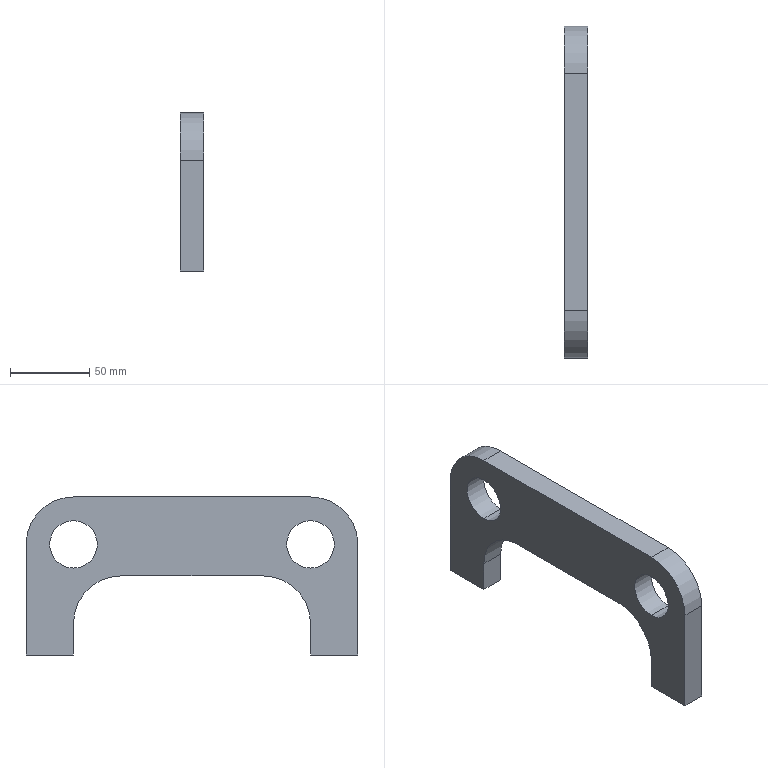Part | SolidWorks | features Cut 1, Extrusion 1 | 1 solid | 18 faces | box 15 x 210 x 100 mm | volume 181294 mm3 | plane 10 | cylinder 8 | commonest cylinder face diameters 30 x4 60 x4
STEP:
#1=CARTESIAN_POINT('',(-215.412,-13.,55.));
#2=VERTEX_POINT('',#1);
#3=CARTESIAN_POINT('',(-215.412,-13.,85.));
#4=VERTEX_POINT('',#3);
#5=CARTESIAN_POINT('',(-215.412,-13.,70.));
#6=DIRECTION('',(-1.,0.,0.));
#7=DIRECTION('',(0.,0.,1.));
#8=AXIS2_PLACEMENT_3D('',#5,#6,#7);
#9=CIRCLE('',#8,15.);
#10=EDGE_CURVE('',#2,#4,#9,.T.);
#11=ORIENTED_EDGE('',*,*,#10,.F.);
#12=CARTESIAN_POINT('',(-230.412,-13.,55.));
#13=VERTEX_POINT('',#12);
#14=CARTESIAN_POINT('',(-215.412,-13.,55.));
#15=DIRECTION('',(-1.,0.,0.));
#16=VECTOR('',#15,1000.);
#17=LINE('',#14,#16);
#18=EDGE_CURVE('',#2,#13,#17,.T.);
#19=ORIENTED_EDGE('',*,*,#18,.T.);
#20=CARTESIAN_POINT('',(-230.412,-13.,85.));
#21=VERTEX_POINT('',#20);
#22=CARTESIAN_POINT('',(-230.412,-13.,70.));
#23=DIRECTION('',(-1.,0.,0.));
#24=DIRECTION('',(0.,0.,1.));
#25=AXIS2_PLACEMENT_3D('',#22,#23,#24);
#26=CIRCLE('',#25,15.);
#27=EDGE_CURVE('',#13,#21,#26,.T.);
#28=ORIENTED_EDGE('',*,*,#27,.T.);
#29=CARTESIAN_POINT('',(-215.412,-13.,85.));
#30=DIRECTION('',(-1.,0.,0.));
#31=VECTOR('',#30,1000.);
#32=LINE('',#29,#31);
#33=EDGE_CURVE('',#4,#21,#32,.T.);
#34=ORIENTED_EDGE('',*,*,#33,.F.);
#35=EDGE_LOOP('',(#11,#19,#28,#34));
#36=FACE_OUTER_BOUND('',#35,.T.);
#37=CARTESIAN_POINT('',(-215.412,-13.,70.));
#38=DIRECTION('',(-1.,0.,0.));
#39=DIRECTION('',(0.,0.,1.));
#40=AXIS2_PLACEMENT_3D('',#37,#38,#39);
#41=CYLINDRICAL_SURFACE('',#40,15.);
#42=ADVANCED_FACE('',(#36),#41,.F.);
#43=CARTESIAN_POINT('',(-215.412,137.,55.));
#44=VERTEX_POINT('',#43);
#45=CARTESIAN_POINT('',(-215.412,137.,85.));
#46=VERTEX_POINT('',#45);
#47=CARTESIAN_POINT('',(-215.412,137.,70.));
#48=DIRECTION('',(-1.,0.,0.));
#49=DIRECTION('',(0.,0.,1.));
#50=AXIS2_PLACEMENT_3D('',#47,#48,#49);
#51=CIRCLE('',#50,15.);
#52=EDGE_CURVE('',#44,#46,#51,.T.);
#53=ORIENTED_EDGE('',*,*,#52,.F.);
#54=CARTESIAN_POINT('',(-230.412,137.,55.));
#55=VERTEX_POINT('',#54);
#56=CARTESIAN_POINT('',(-215.412,137.,55.));
#57=DIRECTION('',(-1.,0.,0.));
#58=VECTOR('',#57,1000.);
#59=LINE('',#56,#58);
#60=EDGE_CURVE('',#44,#55,#59,.T.);
#61=ORIENTED_EDGE('',*,*,#60,.T.);
#62=CARTESIAN_POINT('',(-230.412,137.,85.));
#63=VERTEX_POINT('',#62);
#64=CARTESIAN_POINT('',(-230.412,137.,70.));
#65=DIRECTION('',(-1.,0.,0.));
#66=DIRECTION('',(0.,0.,1.));
#67=AXIS2_PLACEMENT_3D('',#64,#65,#66);
#68=CIRCLE('',#67,15.);
#69=EDGE_CURVE('',#55,#63,#68,.T.);
#70=ORIENTED_EDGE('',*,*,#69,.T.);
#71=CARTESIAN_POINT('',(-215.412,137.,85.));
#72=DIRECTION('',(-1.,0.,0.));
#73=VECTOR('',#72,1000.);
#74=LINE('',#71,#73);
#75=EDGE_CURVE('',#46,#63,#74,.T.);
#76=ORIENTED_EDGE('',*,*,#75,.F.);
#77=EDGE_LOOP('',(#53,#61,#70,#76));
#78=FACE_OUTER_BOUND('',#77,.T.);
#79=CARTESIAN_POINT('',(-215.412,137.,70.));
#80=DIRECTION('',(-1.,0.,0.));
#81=DIRECTION('',(0.,0.,1.));
#82=AXIS2_PLACEMENT_3D('',#79,#80,#81);
#83=CYLINDRICAL_SURFACE('',#82,15.);
#84=ADVANCED_FACE('',(#78),#83,.F.);
#85=CARTESIAN_POINT('',(-230.412,-13.,0.));
#86=VERTEX_POINT('',#85);
#87=CARTESIAN_POINT('',(-230.412,-43.,0.));
#88=VERTEX_POINT('',#87);
#89=CARTESIAN_POINT('',(-230.412,-13.,0.));
#90=DIRECTION('',(0.,-1.,0.));
#91=VECTOR('',#90,1000.);
#92=LINE('',#89,#91);
#93=EDGE_CURVE('',#86,#88,#92,.T.);
#94=ORIENTED_EDGE('',*,*,#93,.F.);
#95=CARTESIAN_POINT('',(-215.412,-13.,0.));
#96=VERTEX_POINT('',#95);
#97=CARTESIAN_POINT('',(-463.006,-13.,0.));
#98=DIRECTION('',(1.,0.,0.));
#99=VECTOR('',#98,1000.);
#100=LINE('',#97,#99);
#101=EDGE_CURVE('',#86,#96,#100,.T.);
#102=ORIENTED_EDGE('',*,*,#101,.T.);
#103=CARTESIAN_POINT('',(-215.412,-43.,0.));
#104=VERTEX_POINT('',#103);
#105=CARTESIAN_POINT('',(-215.412,-13.,0.));
#106=DIRECTION('',(0.,-1.,0.));
#107=VECTOR('',#106,1000.);
#108=LINE('',#105,#107);
#109=EDGE_CURVE('',#96,#104,#108,.T.);
#110=ORIENTED_EDGE('',*,*,#109,.T.);
#111=CARTESIAN_POINT('',(-463.006,-43.,0.));
#112=DIRECTION('',(1.,0.,0.));
#113=VECTOR('',#112,1000.);
#114=LINE('',#111,#113);
#115=EDGE_CURVE('',#88,#104,#114,.T.);
#116=ORIENTED_EDGE('',*,*,#115,.F.);
#117=EDGE_LOOP('',(#94,#102,#110,#116));
#118=FACE_OUTER_BOUND('',#117,.T.);
#119=CARTESIAN_POINT('',(-463.006,-13.,0.));
#120=DIRECTION('',(0.,0.,1.));
#121=DIRECTION('',(1.,0.,0.));
#122=AXIS2_PLACEMENT_3D('',#119,#120,#121);
#123=PLANE('',#122);
#124=ADVANCED_FACE('',(#118),#123,.F.);
#125=CARTESIAN_POINT('',(-230.412,-43.,70.));
#126=VERTEX_POINT('',#125);
#127=CARTESIAN_POINT('',(-230.412,-43.,70.));
#128=DIRECTION('',(0.,0.,1.));
#129=VECTOR('',#128,1000.);
#130=LINE('',#127,#129);
#131=EDGE_CURVE('',#88,#126,#130,.T.);
#132=ORIENTED_EDGE('',*,*,#131,.F.);
#133=ORIENTED_EDGE('',*,*,#115,.T.);
#134=CARTESIAN_POINT('',(-215.412,-43.,70.));
#135=VERTEX_POINT('',#134);
#136=CARTESIAN_POINT('',(-215.412,-43.,70.));
#137=DIRECTION('',(0.,0.,1.));
#138=VECTOR('',#137,1000.);
#139=LINE('',#136,#138);
#140=EDGE_CURVE('',#104,#135,#139,.T.);
#141=ORIENTED_EDGE('',*,*,#140,.T.);
#142=CARTESIAN_POINT('',(-463.006,-43.,70.));
#143=DIRECTION('',(1.,0.,0.));
#144=VECTOR('',#143,1000.);
#145=LINE('',#142,#144);
#146=EDGE_CURVE('',#126,#135,#145,.T.);
#147=ORIENTED_EDGE('',*,*,#146,.F.);
#148=EDGE_LOOP('',(#132,#133,#141,#147));
#149=FACE_OUTER_BOUND('',#148,.T.);
#150=CARTESIAN_POINT('',(-463.006,-43.,70.));
#151=DIRECTION('',(0.,1.,0.));
#152=DIRECTION('',(0.,0.,1.));
#153=AXIS2_PLACEMENT_3D('',#150,#151,#152);
#154=PLANE('',#153);
#155=ADVANCED_FACE('',(#149),#154,.F.);
#156=CARTESIAN_POINT('',(-230.412,-13.,100.));
#157=VERTEX_POINT('',#156);
#158=CARTESIAN_POINT('',(-230.412,-13.,70.));
#159=DIRECTION('',(-1.,0.,0.));
#160=DIRECTION('',(0.,0.,1.));
#161=AXIS2_PLACEMENT_3D('',#158,#159,#160);
#162=CIRCLE('',#161,30.);
#163=EDGE_CURVE('',#126,#157,#162,.T.);
#164=ORIENTED_EDGE('',*,*,#163,.F.);
#165=ORIENTED_EDGE('',*,*,#146,.T.);
#166=CARTESIAN_POINT('',(-215.412,-13.,100.));
#167=VERTEX_POINT('',#166);
#168=CARTESIAN_POINT('',(-215.412,-13.,70.));
#169=DIRECTION('',(-1.,0.,0.));
#170=DIRECTION('',(0.,0.,-1.));
#171=AXIS2_PLACEMENT_3D('',#168,#169,#170);
#172=CIRCLE('',#171,30.);
#173=EDGE_CURVE('',#135,#167,#172,.T.);
#174=ORIENTED_EDGE('',*,*,#173,.T.);
#175=CARTESIAN_POINT('',(-463.006,-13.,100.));
#176=DIRECTION('',(1.,0.,0.));
#177=VECTOR('',#176,1000.);
#178=LINE('',#175,#177);
#179=EDGE_CURVE('',#157,#167,#178,.T.);
#180=ORIENTED_EDGE('',*,*,#179,.F.);
#181=EDGE_LOOP('',(#164,#165,#174,#180));
#182=FACE_OUTER_BOUND('',#181,.T.);
#183=CARTESIAN_POINT('',(-463.006,-13.,70.));
#184=DIRECTION('',(1.,0.,0.));
#185=DIRECTION('',(0.,0.,-1.));
#186=AXIS2_PLACEMENT_3D('',#183,#184,#185);
#187=CYLINDRICAL_SURFACE('',#186,30.);
#188=ADVANCED_FACE('',(#182),#187,.T.);
#189=CARTESIAN_POINT('',(-230.412,137.,100.));
#190=VERTEX_POINT('',#189);
#191=CARTESIAN_POINT('',(-230.412,137.,100.));
#192=DIRECTION('',(0.,1.,0.));
#193=VECTOR('',#192,1000.);
#194=LINE('',#191,#193);
#195=EDGE_CURVE('',#157,#190,#194,.T.);
#196=ORIENTED_EDGE('',*,*,#195,.F.);
#197=ORIENTED_EDGE('',*,*,#179,.T.);
#198=CARTESIAN_POINT('',(-215.412,137.,100.));
#199=VERTEX_POINT('',#198);
#200=CARTESIAN_POINT('',(-215.412,137.,100.));
#201=DIRECTION('',(0.,1.,0.));
#202=VECTOR('',#201,1000.);
#203=LINE('',#200,#202);
#204=EDGE_CURVE('',#167,#199,#203,.T.);
#205=ORIENTED_EDGE('',*,*,#204,.T.);
#206=CARTESIAN_POINT('',(-463.006,137.,100.));
#207=DIRECTION('',(1.,0.,0.));
#208=VECTOR('',#207,1000.);
#209=LINE('',#206,#208);
#210=EDGE_CURVE('',#190,#199,#209,.T.);
#211=ORIENTED_EDGE('',*,*,#210,.F.);
#212=EDGE_LOOP('',(#196,#197,#205,#211));
#213=FACE_OUTER_BOUND('',#212,.T.);
#214=CARTESIAN_POINT('',(-463.006,137.,100.));
#215=DIRECTION('',(0.,0.,-1.));
#216=DIRECTION('',(-1.,0.,0.));
#217=AXIS2_PLACEMENT_3D('',#214,#215,#216);
#218=PLANE('',#217);
#219=ADVANCED_FACE('',(#213),#218,.F.);
#220=CARTESIAN_POINT('',(-230.412,167.,70.));
#221=VERTEX_POINT('',#220);
#222=CARTESIAN_POINT('',(-230.412,137.,70.));
#223=DIRECTION('',(-1.,0.,0.));
#224=DIRECTION('',(0.,0.,1.));
#225=AXIS2_PLACEMENT_3D('',#222,#223,#224);
#226=CIRCLE('',#225,30.);
#227=EDGE_CURVE('',#190,#221,#226,.T.);
#228=ORIENTED_EDGE('',*,*,#227,.F.);
#229=ORIENTED_EDGE('',*,*,#210,.T.);
#230=CARTESIAN_POINT('',(-215.412,167.,70.));
#231=VERTEX_POINT('',#230);
#232=CARTESIAN_POINT('',(-215.412,137.,70.));
#233=DIRECTION('',(-1.,0.,0.));
#234=DIRECTION('',(0.,0.,-1.));
#235=AXIS2_PLACEMENT_3D('',#232,#233,#234);
#236=CIRCLE('',#235,30.);
#237=EDGE_CURVE('',#199,#231,#236,.T.);
#238=ORIENTED_EDGE('',*,*,#237,.T.);
#239=CARTESIAN_POINT('',(-463.006,167.,70.));
#240=DIRECTION('',(1.,0.,0.));
#241=VECTOR('',#240,1000.);
#242=LINE('',#239,#241);
#243=EDGE_CURVE('',#221,#231,#242,.T.);
#244=ORIENTED_EDGE('',*,*,#243,.F.);
#245=EDGE_LOOP('',(#228,#229,#238,#244));
#246=FACE_OUTER_BOUND('',#245,.T.);
#247=CARTESIAN_POINT('',(-463.006,137.,70.));
#248=DIRECTION('',(1.,0.,0.));
#249=DIRECTION('',(0.,0.,-1.));
#250=AXIS2_PLACEMENT_3D('',#247,#248,#249);
#251=CYLINDRICAL_SURFACE('',#250,30.);
#252=ADVANCED_FACE('',(#246),#251,.T.);
#253=CARTESIAN_POINT('',(-230.412,167.,0.));
#254=VERTEX_POINT('',#253);
#255=CARTESIAN_POINT('',(-230.412,167.,0.));
#256=DIRECTION('',(0.,0.,-1.));
#257=VECTOR('',#256,1000.);
#258=LINE('',#255,#257);
#259=EDGE_CURVE('',#221,#254,#258,.T.);
#260=ORIENTED_EDGE('',*,*,#259,.F.);
#261=ORIENTED_EDGE('',*,*,#243,.T.);
#262=CARTESIAN_POINT('',(-215.412,167.,0.));
#263=VERTEX_POINT('',#262);
#264=CARTESIAN_POINT('',(-215.412,167.,0.));
#265=DIRECTION('',(0.,0.,-1.));
#266=VECTOR('',#265,1000.);
#267=LINE('',#264,#266);
#268=EDGE_CURVE('',#231,#263,#267,.T.);
#269=ORIENTED_EDGE('',*,*,#268,.T.);
#270=CARTESIAN_POINT('',(-463.006,167.,0.));
#271=DIRECTION('',(1.,0.,0.));
#272=VECTOR('',#271,1000.);
#273=LINE('',#270,#272);
#274=EDGE_CURVE('',#254,#263,#273,.T.);
#275=ORIENTED_EDGE('',*,*,#274,.F.);
#276=EDGE_LOOP('',(#260,#261,#269,#275));
#277=FACE_OUTER_BOUND('',#276,.T.);
#278=CARTESIAN_POINT('',(-463.006,167.,0.));
#279=DIRECTION('',(0.,-1.,0.));
#280=DIRECTION('',(1.,0.,0.));
#281=AXIS2_PLACEMENT_3D('',#278,#279,#280);
#282=PLANE('',#281);
#283=ADVANCED_FACE('',(#277),#282,.F.);
#284=CARTESIAN_POINT('',(-230.412,137.,0.));
#285=VERTEX_POINT('',#284);
#286=CARTESIAN_POINT('',(-230.412,137.,0.));
#287=DIRECTION('',(0.,-1.,0.));
#288=VECTOR('',#287,1000.);
#289=LINE('',#286,#288);
#290=EDGE_CURVE('',#254,#285,#289,.T.);
#291=ORIENTED_EDGE('',*,*,#290,.F.);
#292=ORIENTED_EDGE('',*,*,#274,.T.);
#293=CARTESIAN_POINT('',(-215.412,137.,0.));
#294=VERTEX_POINT('',#293);
#295=CARTESIAN_POINT('',(-215.412,137.,0.));
#296=DIRECTION('',(0.,-1.,0.));
#297=VECTOR('',#296,1000.);
#298=LINE('',#295,#297);
#299=EDGE_CURVE('',#263,#294,#298,.T.);
#300=ORIENTED_EDGE('',*,*,#299,.T.);
#301=CARTESIAN_POINT('',(-463.006,137.,0.));
#302=DIRECTION('',(1.,0.,0.));
#303=VECTOR('',#302,1000.);
#304=LINE('',#301,#303);
#305=EDGE_CURVE('',#285,#294,#304,.T.);
#306=ORIENTED_EDGE('',*,*,#305,.F.);
#307=EDGE_LOOP('',(#291,#292,#300,#306));
#308=FACE_OUTER_BOUND('',#307,.T.);
#309=CARTESIAN_POINT('',(-463.006,137.,0.));
#310=DIRECTION('',(0.,0.,1.));
#311=DIRECTION('',(1.,0.,0.));
#312=AXIS2_PLACEMENT_3D('',#309,#310,#311);
#313=PLANE('',#312);
#314=ADVANCED_FACE('',(#308),#313,.F.);
#315=CARTESIAN_POINT('',(-230.412,137.,20.));
#316=VERTEX_POINT('',#315);
#317=CARTESIAN_POINT('',(-230.412,137.,20.));
#318=DIRECTION('',(0.,0.,1.));
#319=VECTOR('',#318,1000.);
#320=LINE('',#317,#319);
#321=EDGE_CURVE('',#285,#316,#320,.T.);
#322=ORIENTED_EDGE('',*,*,#321,.F.);
#323=ORIENTED_EDGE('',*,*,#305,.T.);
#324=CARTESIAN_POINT('',(-215.412,137.,20.));
#325=VERTEX_POINT('',#324);
#326=CARTESIAN_POINT('',(-215.412,137.,20.));
#327=DIRECTION('',(0.,0.,1.));
#328=VECTOR('',#327,1000.);
#329=LINE('',#326,#328);
#330=EDGE_CURVE('',#294,#325,#329,.T.);
#331=ORIENTED_EDGE('',*,*,#330,.T.);
#332=CARTESIAN_POINT('',(-463.006,137.,20.));
#333=DIRECTION('',(1.,0.,0.));
#334=VECTOR('',#333,1000.);
#335=LINE('',#332,#334);
#336=EDGE_CURVE('',#316,#325,#335,.T.);
#337=ORIENTED_EDGE('',*,*,#336,.F.);
#338=EDGE_LOOP('',(#322,#323,#331,#337));
#339=FACE_OUTER_BOUND('',#338,.T.);
#340=CARTESIAN_POINT('',(-463.006,137.,20.));
#341=DIRECTION('',(0.,1.,0.));
#342=DIRECTION('',(-1.,0.,0.));
#343=AXIS2_PLACEMENT_3D('',#340,#341,#342);
#344=PLANE('',#343);
#345=ADVANCED_FACE('',(#339),#344,.F.);
#346=CARTESIAN_POINT('',(-230.412,107.,50.));
#347=VERTEX_POINT('',#346);
#348=CARTESIAN_POINT('',(-230.412,107.,20.));
#349=DIRECTION('',(1.,0.,0.));
#350=DIRECTION('',(0.,0.,1.));
#351=AXIS2_PLACEMENT_3D('',#348,#349,#350);
#352=CIRCLE('',#351,30.);
#353=EDGE_CURVE('',#316,#347,#352,.T.);
#354=ORIENTED_EDGE('',*,*,#353,.F.);
#355=ORIENTED_EDGE('',*,*,#336,.T.);
#356=CARTESIAN_POINT('',(-215.412,107.,50.));
#357=VERTEX_POINT('',#356);
#358=CARTESIAN_POINT('',(-215.412,107.,20.));
#359=DIRECTION('',(1.,0.,0.));
#360=DIRECTION('',(0.,0.,1.));
#361=AXIS2_PLACEMENT_3D('',#358,#359,#360);
#362=CIRCLE('',#361,30.);
#363=EDGE_CURVE('',#325,#357,#362,.T.);
#364=ORIENTED_EDGE('',*,*,#363,.T.);
#365=CARTESIAN_POINT('',(-463.006,107.,50.));
#366=DIRECTION('',(1.,0.,0.));
#367=VECTOR('',#366,1000.);
#368=LINE('',#365,#367);
#369=EDGE_CURVE('',#347,#357,#368,.T.);
#370=ORIENTED_EDGE('',*,*,#369,.F.);
#371=EDGE_LOOP('',(#354,#355,#364,#370));
#372=FACE_OUTER_BOUND('',#371,.T.);
#373=CARTESIAN_POINT('',(-463.006,107.,20.));
#374=DIRECTION('',(1.,0.,0.));
#375=DIRECTION('',(0.,0.,-1.));
#376=AXIS2_PLACEMENT_3D('',#373,#374,#375);
#377=CYLINDRICAL_SURFACE('',#376,30.);
#378=ADVANCED_FACE('',(#372),#377,.F.);
#379=CARTESIAN_POINT('',(-230.412,17.,50.));
#380=VERTEX_POINT('',#379);
#381=CARTESIAN_POINT('',(-230.412,17.,50.));
#382=DIRECTION('',(0.,-1.,0.));
#383=VECTOR('',#382,1000.);
#384=LINE('',#381,#383);
#385=EDGE_CURVE('',#347,#380,#384,.T.);
#386=ORIENTED_EDGE('',*,*,#385,.F.);
#387=ORIENTED_EDGE('',*,*,#369,.T.);
#388=CARTESIAN_POINT('',(-215.412,17.,50.));
#389=VERTEX_POINT('',#388);
#390=CARTESIAN_POINT('',(-215.412,17.,50.));
#391=DIRECTION('',(0.,-1.,0.));
#392=VECTOR('',#391,1000.);
#393=LINE('',#390,#392);
#394=EDGE_CURVE('',#357,#389,#393,.T.);
#395=ORIENTED_EDGE('',*,*,#394,.T.);
#396=CARTESIAN_POINT('',(-463.006,17.,50.));
#397=DIRECTION('',(1.,0.,0.));
#398=VECTOR('',#397,1000.);
#399=LINE('',#396,#398);
#400=EDGE_CURVE('',#380,#389,#399,.T.);
#401=ORIENTED_EDGE('',*,*,#400,.F.);
#402=EDGE_LOOP('',(#386,#387,#395,#401));
#403=FACE_OUTER_BOUND('',#402,.T.);
#404=CARTESIAN_POINT('',(-463.006,17.,50.));
#405=DIRECTION('',(0.,0.,1.));
#406=DIRECTION('',(1.,0.,0.));
#407=AXIS2_PLACEMENT_3D('',#404,#405,#406);
#408=PLANE('',#407);
#409=ADVANCED_FACE('',(#403),#408,.F.);
#410=CARTESIAN_POINT('',(-230.412,-13.,20.));
#411=VERTEX_POINT('',#410);
#412=CARTESIAN_POINT('',(-230.412,17.,20.));
#413=DIRECTION('',(1.,0.,0.));
#414=DIRECTION('',(0.,0.,1.));
#415=AXIS2_PLACEMENT_3D('',#412,#413,#414);
#416=CIRCLE('',#415,30.);
#417=EDGE_CURVE('',#380,#411,#416,.T.);
#418=ORIENTED_EDGE('',*,*,#417,.F.);
#419=ORIENTED_EDGE('',*,*,#400,.T.);
#420=CARTESIAN_POINT('',(-215.412,-13.,20.));
#421=VERTEX_POINT('',#420);
#422=CARTESIAN_POINT('',(-215.412,17.,20.));
#423=DIRECTION('',(1.,0.,0.));
#424=DIRECTION('',(0.,0.,1.));
#425=AXIS2_PLACEMENT_3D('',#422,#423,#424);
#426=CIRCLE('',#425,30.);
#427=EDGE_CURVE('',#389,#421,#426,.T.);
#428=ORIENTED_EDGE('',*,*,#427,.T.);
#429=CARTESIAN_POINT('',(-463.006,-13.,20.));
#430=DIRECTION('',(1.,0.,0.));
#431=VECTOR('',#430,1000.);
#432=LINE('',#429,#431);
#433=EDGE_CURVE('',#411,#421,#432,.T.);
#434=ORIENTED_EDGE('',*,*,#433,.F.);
#435=EDGE_LOOP('',(#418,#419,#428,#434));
#436=FACE_OUTER_BOUND('',#435,.T.);
#437=CARTESIAN_POINT('',(-463.006,17.,20.));
#438=DIRECTION('',(1.,0.,0.));
#439=DIRECTION('',(0.,0.,-1.));
#440=AXIS2_PLACEMENT_3D('',#437,#438,#439);
#441=CYLINDRICAL_SURFACE('',#440,30.);
#442=ADVANCED_FACE('',(#436),#441,.F.);
#443=CARTESIAN_POINT('',(-230.412,-13.,0.));
#444=DIRECTION('',(0.,0.,-1.));
#445=VECTOR('',#444,1000.);
#446=LINE('',#443,#445);
#447=EDGE_CURVE('',#411,#86,#446,.T.);
#448=ORIENTED_EDGE('',*,*,#447,.F.);
#449=ORIENTED_EDGE('',*,*,#433,.T.);
#450=CARTESIAN_POINT('',(-215.412,-13.,0.));
#451=DIRECTION('',(0.,0.,-1.));
#452=VECTOR('',#451,1000.);
#453=LINE('',#450,#452);
#454=EDGE_CURVE('',#421,#96,#453,.T.);
#455=ORIENTED_EDGE('',*,*,#454,.T.);
#456=ORIENTED_EDGE('',*,*,#101,.F.);
#457=EDGE_LOOP('',(#448,#449,#455,#456));
#458=FACE_OUTER_BOUND('',#457,.T.);
#459=CARTESIAN_POINT('',(-463.006,-13.,0.));
#460=DIRECTION('',(0.,-1.,0.));
#461=DIRECTION('',(1.,0.,0.));
#462=AXIS2_PLACEMENT_3D('',#459,#460,#461);
#463=PLANE('',#462);
#464=ADVANCED_FACE('',(#458),#463,.F.);
#465=CARTESIAN_POINT('',(-215.412,-13.,70.));
#466=DIRECTION('',(-1.,0.,0.));
#467=DIRECTION('',(0.,0.,1.));
#468=AXIS2_PLACEMENT_3D('',#465,#466,#467);
#469=CIRCLE('',#468,15.);
#470=EDGE_CURVE('',#4,#2,#469,.T.);
#471=ORIENTED_EDGE('',*,*,#470,.T.);
#472=ORIENTED_EDGE('',*,*,#10,.T.);
#473=EDGE_LOOP('',(#471,#472));
#474=FACE_BOUND('',#473,.T.);
#475=CARTESIAN_POINT('',(-215.412,137.,70.));
#476=DIRECTION('',(-1.,0.,0.));
#477=DIRECTION('',(0.,0.,1.));
#478=AXIS2_PLACEMENT_3D('',#475,#476,#477);
#479=CIRCLE('',#478,15.);
#480=EDGE_CURVE('',#46,#44,#479,.T.);
#481=ORIENTED_EDGE('',*,*,#480,.T.);
#482=ORIENTED_EDGE('',*,*,#52,.T.);
#483=EDGE_LOOP('',(#481,#482));
#484=FACE_BOUND('',#483,.T.);
#485=ORIENTED_EDGE('',*,*,#109,.F.);
#486=ORIENTED_EDGE('',*,*,#454,.F.);
#487=ORIENTED_EDGE('',*,*,#427,.F.);
#488=ORIENTED_EDGE('',*,*,#394,.F.);
#489=ORIENTED_EDGE('',*,*,#363,.F.);
#490=ORIENTED_EDGE('',*,*,#330,.F.);
#491=ORIENTED_EDGE('',*,*,#299,.F.);
#492=ORIENTED_EDGE('',*,*,#268,.F.);
#493=ORIENTED_EDGE('',*,*,#237,.F.);
#494=ORIENTED_EDGE('',*,*,#204,.F.);
#495=ORIENTED_EDGE('',*,*,#173,.F.);
#496=ORIENTED_EDGE('',*,*,#140,.F.);
#497=EDGE_LOOP('',(#485,#486,#487,#488,#489,#490,#491,#492,#493,#494,#495,#496));
#498=FACE_OUTER_BOUND('',#497,.T.);
#499=CARTESIAN_POINT('',(-215.412,-13.,70.));
#500=DIRECTION('',(1.,0.,0.));
#501=DIRECTION('',(0.,0.,-1.));
#502=AXIS2_PLACEMENT_3D('',#499,#500,#501);
#503=PLANE('',#502);
#504=ADVANCED_FACE('',(#474,#484,#498),#503,.T.);
#505=CARTESIAN_POINT('',(-230.412,-13.,70.));
#506=DIRECTION('',(-1.,0.,0.));
#507=DIRECTION('',(0.,0.,1.));
#508=AXIS2_PLACEMENT_3D('',#505,#506,#507);
#509=CIRCLE('',#508,15.);
#510=EDGE_CURVE('',#21,#13,#509,.T.);
#511=ORIENTED_EDGE('',*,*,#510,.F.);
#512=ORIENTED_EDGE('',*,*,#27,.F.);
#513=EDGE_LOOP('',(#511,#512));
#514=FACE_BOUND('',#513,.T.);
#515=CARTESIAN_POINT('',(-230.412,137.,70.));
#516=DIRECTION('',(-1.,0.,0.));
#517=DIRECTION('',(0.,0.,1.));
#518=AXIS2_PLACEMENT_3D('',#515,#516,#517);
#519=CIRCLE('',#518,15.);
#520=EDGE_CURVE('',#63,#55,#519,.T.);
#521=ORIENTED_EDGE('',*,*,#520,.F.);
#522=ORIENTED_EDGE('',*,*,#69,.F.);
#523=EDGE_LOOP('',(#521,#522));
#524=FACE_BOUND('',#523,.T.);
#525=ORIENTED_EDGE('',*,*,#447,.T.);
#526=ORIENTED_EDGE('',*,*,#93,.T.);
#527=ORIENTED_EDGE('',*,*,#131,.T.);
#528=ORIENTED_EDGE('',*,*,#163,.T.);
#529=ORIENTED_EDGE('',*,*,#195,.T.);
#530=ORIENTED_EDGE('',*,*,#227,.T.);
#531=ORIENTED_EDGE('',*,*,#259,.T.);
#532=ORIENTED_EDGE('',*,*,#290,.T.);
#533=ORIENTED_EDGE('',*,*,#321,.T.);
#534=ORIENTED_EDGE('',*,*,#353,.T.);
#535=ORIENTED_EDGE('',*,*,#385,.T.);
#536=ORIENTED_EDGE('',*,*,#417,.T.);
#537=EDGE_LOOP('',(#525,#526,#527,#528,#529,#530,#531,#532,#533,#534,#535,#536));
#538=FACE_OUTER_BOUND('',#537,.T.);
#539=CARTESIAN_POINT('',(-230.412,-43.,0.));
#540=DIRECTION('',(-1.,0.,0.));
#541=DIRECTION('',(0.,0.,-1.));
#542=AXIS2_PLACEMENT_3D('',#539,#540,#541);
#543=PLANE('',#542);
#544=ADVANCED_FACE('',(#514,#524,#538),#543,.T.);
#545=ORIENTED_EDGE('',*,*,#60,.F.);
#546=ORIENTED_EDGE('',*,*,#480,.F.);
#547=ORIENTED_EDGE('',*,*,#75,.T.);
#548=ORIENTED_EDGE('',*,*,#520,.T.);
#549=EDGE_LOOP('',(#545,#546,#547,#548));
#550=FACE_OUTER_BOUND('',#549,.T.);
#551=CARTESIAN_POINT('',(-215.412,137.,70.));
#552=DIRECTION('',(-1.,0.,0.));
#553=DIRECTION('',(0.,0.,1.));
#554=AXIS2_PLACEMENT_3D('',#551,#552,#553);
#555=CYLINDRICAL_SURFACE('',#554,15.);
#556=ADVANCED_FACE('',(#550),#555,.F.);
#557=ORIENTED_EDGE('',*,*,#18,.F.);
#558=ORIENTED_EDGE('',*,*,#470,.F.);
#559=ORIENTED_EDGE('',*,*,#33,.T.);
#560=ORIENTED_EDGE('',*,*,#510,.T.);
#561=EDGE_LOOP('',(#557,#558,#559,#560));
#562=FACE_OUTER_BOUND('',#561,.T.);
#563=CARTESIAN_POINT('',(-215.412,-13.,70.));
#564=DIRECTION('',(-1.,0.,0.));
#565=DIRECTION('',(0.,0.,1.));
#566=AXIS2_PLACEMENT_3D('',#563,#564,#565);
#567=CYLINDRICAL_SURFACE('',#566,15.);
#568=ADVANCED_FACE('',(#562),#567,.F.);
#569=CLOSED_SHELL('',(#42,#84,#124,#155,#188,#219,#252,#283,#314,#345,#378,#409,#442,#464,#504,#544,#556,#568));
#570=MANIFOLD_SOLID_BREP('',#569);
#571=CARTESIAN_POINT('',(0.,0.,0.));
#572=DIRECTION('',(0.,0.,1.));
#573=DIRECTION('',(1.,0.,0.));
#574=AXIS2_PLACEMENT_3D('',#571,#572,#573);
#575=(LENGTH_UNIT()NAMED_UNIT(*)SI_UNIT(.MILLI.,.METRE.));
#576=UNCERTAINTY_MEASURE_WITH_UNIT(LENGTH_MEASURE(0.00001),#575,'','');
#577=(NAMED_UNIT(*)PLANE_ANGLE_UNIT()SI_UNIT($,.RADIAN.));
#578=(NAMED_UNIT(*)SI_UNIT($,.STERADIAN.)SOLID_ANGLE_UNIT());
#579=(GEOMETRIC_REPRESENTATION_CONTEXT(3)GLOBAL_UNCERTAINTY_ASSIGNED_CONTEXT((#576))GLOBAL_UNIT_ASSIGNED_CONTEXT((#575,#577,#578))REPRESENTATION_CONTEXT('',''));
#580=ADVANCED_BREP_SHAPE_REPRESENTATION('',(#570,#574),#579);